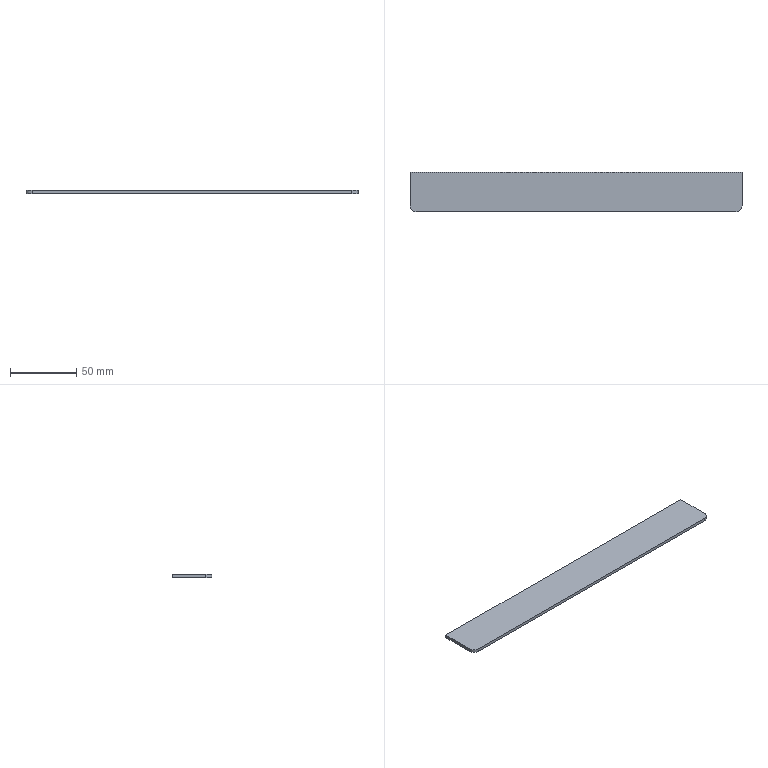Part | STEP file | [04]-7 | 1 solid | 8 faces | box 250 x 30 x 2.3 mm | volume 17229 mm3 | plane 6 | cylinder 2 | commonest cylinder face diameters 9.2 x2
STEP:
#1=CARTESIAN_POINT('',(0.,0.,0.));
#2=DIRECTION('',(0.,0.,1.));
#3=DIRECTION('',(1.,0.,0.));
#4=AXIS2_PLACEMENT_3D('',#1,#2,#3);
#5=CARTESIAN_POINT('',(0.,-25.4,0.));
#6=VERTEX_POINT('',#5);
#7=CARTESIAN_POINT('',(0.,0.,0.));
#8=VERTEX_POINT('',#7);
#9=CARTESIAN_POINT('',(0.,-15.,0.));
#10=DIRECTION('',(0.,1.,0.));
#11=VECTOR('',#10,1.);
#12=LINE('',#9,#11);
#13=CARTESIAN_POINT('',(125.,-15.,0.));
#14=DIRECTION('',(0.,0.,-1.));
#15=DIRECTION('',(-1.,0.,0.));
#16=AXIS2_PLACEMENT_3D('',#13,#14,#15);
#17=PLANE('',#16);
#18=CARTESIAN_POINT('',(125.,0.));
#19=DIRECTION('',(0.,1.));
#20=VECTOR('',#19,1.);
#21=LINE('',#18,#20);
#22=(GEOMETRIC_REPRESENTATION_CONTEXT(2)PARAMETRIC_REPRESENTATION_CONTEXT()REPRESENTATION_CONTEXT('',''));
#23=DEFINITIONAL_REPRESENTATION('',(#21),#22);
#24=PCURVE('',#17,#23);
#25=CARTESIAN_POINT('',(0.,-15.,2.3));
#26=DIRECTION('',(-1.,0.,0.));
#27=DIRECTION('',(0.,0.,1.));
#28=AXIS2_PLACEMENT_3D('',#25,#26,#27);
#29=PLANE('',#28);
#30=CARTESIAN_POINT('',(-2.3,0.));
#31=DIRECTION('',(0.,1.));
#32=VECTOR('',#31,1.);
#33=LINE('',#30,#32);
#34=(GEOMETRIC_REPRESENTATION_CONTEXT(2)PARAMETRIC_REPRESENTATION_CONTEXT()REPRESENTATION_CONTEXT('',''));
#35=DEFINITIONAL_REPRESENTATION('',(#33),#34);
#36=PCURVE('',#29,#35);
#37=SURFACE_CURVE('',#12,(#24,#36),.PCURVE_S1.);
#38=EDGE_CURVE('',#6,#8,#37,.T.);
#39=ORIENTED_EDGE('',*,*,#38,.T.);
#40=CARTESIAN_POINT('',(250.,0.,0.));
#41=VERTEX_POINT('',#40);
#42=CARTESIAN_POINT('',(125.,0.,0.));
#43=DIRECTION('',(1.,0.,0.));
#44=VECTOR('',#43,1.);
#45=LINE('',#42,#44);
#46=CARTESIAN_POINT('',(0.,15.));
#47=DIRECTION('',(-1.,0.));
#48=VECTOR('',#47,1.);
#49=LINE('',#46,#48);
#50=(GEOMETRIC_REPRESENTATION_CONTEXT(2)PARAMETRIC_REPRESENTATION_CONTEXT()REPRESENTATION_CONTEXT('',''));
#51=DEFINITIONAL_REPRESENTATION('',(#49),#50);
#52=PCURVE('',#17,#51);
#53=CARTESIAN_POINT('',(125.,0.,2.3));
#54=DIRECTION('',(0.,1.,0.));
#55=DIRECTION('',(0.,0.,1.));
#56=AXIS2_PLACEMENT_3D('',#53,#54,#55);
#57=PLANE('',#56);
#58=CARTESIAN_POINT('',(-2.3,0.));
#59=DIRECTION('',(0.,1.));
#60=VECTOR('',#59,1.);
#61=LINE('',#58,#60);
#62=(GEOMETRIC_REPRESENTATION_CONTEXT(2)PARAMETRIC_REPRESENTATION_CONTEXT()REPRESENTATION_CONTEXT('',''));
#63=DEFINITIONAL_REPRESENTATION('',(#61),#62);
#64=PCURVE('',#57,#63);
#65=SURFACE_CURVE('',#45,(#52,#64),.PCURVE_S1.);
#66=EDGE_CURVE('',#8,#41,#65,.T.);
#67=ORIENTED_EDGE('',*,*,#66,.T.);
#68=CARTESIAN_POINT('',(250.,-25.4,0.));
#69=VERTEX_POINT('',#68);
#70=CARTESIAN_POINT('',(250.,-15.,0.));
#71=DIRECTION('',(0.,-1.,0.));
#72=VECTOR('',#71,1.);
#73=LINE('',#70,#72);
#74=CARTESIAN_POINT('',(-125.,0.));
#75=DIRECTION('',(0.,-1.));
#76=VECTOR('',#75,1.);
#77=LINE('',#74,#76);
#78=(GEOMETRIC_REPRESENTATION_CONTEXT(2)PARAMETRIC_REPRESENTATION_CONTEXT()REPRESENTATION_CONTEXT('',''));
#79=DEFINITIONAL_REPRESENTATION('',(#77),#78);
#80=PCURVE('',#17,#79);
#81=CARTESIAN_POINT('',(250.,-15.,2.3));
#82=DIRECTION('',(1.,0.,0.));
#83=DIRECTION('',(0.,0.,-1.));
#84=AXIS2_PLACEMENT_3D('',#81,#82,#83);
#85=PLANE('',#84);
#86=CARTESIAN_POINT('',(2.3,0.));
#87=DIRECTION('',(0.,-1.));
#88=VECTOR('',#87,1.);
#89=LINE('',#86,#88);
#90=(GEOMETRIC_REPRESENTATION_CONTEXT(2)PARAMETRIC_REPRESENTATION_CONTEXT()REPRESENTATION_CONTEXT('',''));
#91=DEFINITIONAL_REPRESENTATION('',(#89),#90);
#92=PCURVE('',#85,#91);
#93=SURFACE_CURVE('',#73,(#80,#92),.PCURVE_S1.);
#94=EDGE_CURVE('',#41,#69,#93,.T.);
#95=ORIENTED_EDGE('',*,*,#94,.T.);
#96=CARTESIAN_POINT('',(245.4,-30.,0.));
#97=VERTEX_POINT('',#96);
#98=CARTESIAN_POINT('',(245.4,-25.4,0.));
#99=DIRECTION('',(0.,0.,1.));
#100=DIRECTION('',(-1.,0.,0.));
#101=AXIS2_PLACEMENT_3D('',#98,#99,#100);
#102=CIRCLE('',#101,4.6);
#103=CARTESIAN_POINT('',(-115.8,-10.4));
#104=CARTESIAN_POINT('',(-115.8,-18.367));
#105=CARTESIAN_POINT('',(-122.7,-14.384));
#106=CARTESIAN_POINT('',(-129.6,-10.4));
#107=CARTESIAN_POINT('',(-122.7,-6.416));
#108=CARTESIAN_POINT('',(-115.8,-2.433));
#109=CARTESIAN_POINT('',(-115.8,-10.4));
#110=(BOUNDED_CURVE()B_SPLINE_CURVE(2,(#103,#104,#105,#106,#107,#108,#109),.UNSPECIFIED.,.T.,.F.)B_SPLINE_CURVE_WITH_KNOTS((1,2,2,2,2,1),(-2.094,0.,2.094,4.189,6.283,8.378),.UNSPECIFIED.)CURVE()GEOMETRIC_REPRESENTATION_ITEM()RATIONAL_B_SPLINE_CURVE((1.,0.5,1.,0.5,1.,0.5,1.))REPRESENTATION_ITEM(''));
#111=(GEOMETRIC_REPRESENTATION_CONTEXT(2)PARAMETRIC_REPRESENTATION_CONTEXT()REPRESENTATION_CONTEXT('',''));
#112=DEFINITIONAL_REPRESENTATION('',(#110),#111);
#113=PCURVE('',#17,#112);
#114=CARTESIAN_POINT('',(245.4,-25.4,2.3));
#115=DIRECTION('',(0.,0.,-1.));
#116=DIRECTION('',(-1.,0.,0.));
#117=AXIS2_PLACEMENT_3D('',#114,#115,#116);
#118=CYLINDRICAL_SURFACE('',#117,4.6);
#119=CARTESIAN_POINT('',(6.283,2.3));
#120=DIRECTION('',(-1.,0.));
#121=VECTOR('',#120,1.);
#122=LINE('',#119,#121);
#123=(GEOMETRIC_REPRESENTATION_CONTEXT(2)PARAMETRIC_REPRESENTATION_CONTEXT()REPRESENTATION_CONTEXT('',''));
#124=DEFINITIONAL_REPRESENTATION('',(#122),#123);
#125=PCURVE('',#118,#124);
#126=SURFACE_CURVE('',#102,(#113,#125),.PCURVE_S1.);
#127=EDGE_CURVE('',#97,#69,#126,.T.);
#128=ORIENTED_EDGE('',*,*,#127,.F.);
#129=CARTESIAN_POINT('',(4.6,-30.,0.));
#130=VERTEX_POINT('',#129);
#131=CARTESIAN_POINT('',(125.,-30.,0.));
#132=DIRECTION('',(-1.,0.,0.));
#133=VECTOR('',#132,1.);
#134=LINE('',#131,#133);
#135=CARTESIAN_POINT('',(0.,-15.));
#136=DIRECTION('',(1.,0.));
#137=VECTOR('',#136,1.);
#138=LINE('',#135,#137);
#139=(GEOMETRIC_REPRESENTATION_CONTEXT(2)PARAMETRIC_REPRESENTATION_CONTEXT()REPRESENTATION_CONTEXT('',''));
#140=DEFINITIONAL_REPRESENTATION('',(#138),#139);
#141=PCURVE('',#17,#140);
#142=CARTESIAN_POINT('',(125.,-30.,2.3));
#143=DIRECTION('',(0.,-1.,0.));
#144=DIRECTION('',(0.,0.,-1.));
#145=AXIS2_PLACEMENT_3D('',#142,#143,#144);
#146=PLANE('',#145);
#147=CARTESIAN_POINT('',(2.3,0.));
#148=DIRECTION('',(0.,-1.));
#149=VECTOR('',#148,1.);
#150=LINE('',#147,#149);
#151=(GEOMETRIC_REPRESENTATION_CONTEXT(2)PARAMETRIC_REPRESENTATION_CONTEXT()REPRESENTATION_CONTEXT('',''));
#152=DEFINITIONAL_REPRESENTATION('',(#150),#151);
#153=PCURVE('',#146,#152);
#154=SURFACE_CURVE('',#134,(#141,#153),.PCURVE_S1.);
#155=EDGE_CURVE('',#97,#130,#154,.T.);
#156=ORIENTED_EDGE('',*,*,#155,.T.);
#157=CARTESIAN_POINT('',(4.6,-25.4,0.));
#158=DIRECTION('',(0.,0.,1.));
#159=DIRECTION('',(-1.,0.,0.));
#160=AXIS2_PLACEMENT_3D('',#157,#158,#159);
#161=CIRCLE('',#160,4.6);
#162=CARTESIAN_POINT('',(125.,-10.4));
#163=CARTESIAN_POINT('',(125.,-18.367));
#164=CARTESIAN_POINT('',(118.1,-14.384));
#165=CARTESIAN_POINT('',(111.2,-10.4));
#166=CARTESIAN_POINT('',(118.1,-6.416));
#167=CARTESIAN_POINT('',(125.,-2.433));
#168=CARTESIAN_POINT('',(125.,-10.4));
#169=(BOUNDED_CURVE()B_SPLINE_CURVE(2,(#162,#163,#164,#165,#166,#167,#168),.UNSPECIFIED.,.T.,.F.)B_SPLINE_CURVE_WITH_KNOTS((1,2,2,2,2,1),(-2.094,0.,2.094,4.189,6.283,8.378),.UNSPECIFIED.)CURVE()GEOMETRIC_REPRESENTATION_ITEM()RATIONAL_B_SPLINE_CURVE((1.,0.5,1.,0.5,1.,0.5,1.))REPRESENTATION_ITEM(''));
#170=(GEOMETRIC_REPRESENTATION_CONTEXT(2)PARAMETRIC_REPRESENTATION_CONTEXT()REPRESENTATION_CONTEXT('',''));
#171=DEFINITIONAL_REPRESENTATION('',(#169),#170);
#172=PCURVE('',#17,#171);
#173=CARTESIAN_POINT('',(4.6,-25.4,2.3));
#174=DIRECTION('',(0.,0.,-1.));
#175=DIRECTION('',(-1.,0.,0.));
#176=AXIS2_PLACEMENT_3D('',#173,#174,#175);
#177=CYLINDRICAL_SURFACE('',#176,4.6);
#178=CARTESIAN_POINT('',(6.283,2.3));
#179=DIRECTION('',(-1.,0.));
#180=VECTOR('',#179,1.);
#181=LINE('',#178,#180);
#182=(GEOMETRIC_REPRESENTATION_CONTEXT(2)PARAMETRIC_REPRESENTATION_CONTEXT()REPRESENTATION_CONTEXT('',''));
#183=DEFINITIONAL_REPRESENTATION('',(#181),#182);
#184=PCURVE('',#177,#183);
#185=SURFACE_CURVE('',#161,(#172,#184),.PCURVE_S1.);
#186=EDGE_CURVE('',#6,#130,#185,.T.);
#187=ORIENTED_EDGE('',*,*,#186,.F.);
#188=EDGE_LOOP('',(#39,#67,#95,#128,#156,#187));
#189=FACE_BOUND('',#188,.T.);
#190=ADVANCED_FACE('',(#189),#17,.T.);
#191=CARTESIAN_POINT('',(0.,0.,2.3));
#192=VERTEX_POINT('',#191);
#193=CARTESIAN_POINT('',(0.,0.,2.3));
#194=DIRECTION('',(0.,0.,-1.));
#195=VECTOR('',#194,1.);
#196=LINE('',#193,#195);
#197=CARTESIAN_POINT('',(0.,-125.));
#198=DIRECTION('',(-1.,0.));
#199=VECTOR('',#198,1.);
#200=LINE('',#197,#199);
#201=(GEOMETRIC_REPRESENTATION_CONTEXT(2)PARAMETRIC_REPRESENTATION_CONTEXT()REPRESENTATION_CONTEXT('',''));
#202=DEFINITIONAL_REPRESENTATION('',(#200),#201);
#203=PCURVE('',#57,#202);
#204=CARTESIAN_POINT('',(0.,15.));
#205=DIRECTION('',(-1.,0.));
#206=VECTOR('',#205,1.);
#207=LINE('',#204,#206);
#208=(GEOMETRIC_REPRESENTATION_CONTEXT(2)PARAMETRIC_REPRESENTATION_CONTEXT()REPRESENTATION_CONTEXT('',''));
#209=DEFINITIONAL_REPRESENTATION('',(#207),#208);
#210=PCURVE('',#29,#209);
#211=SURFACE_CURVE('',#196,(#203,#210),.PCURVE_S1.);
#212=EDGE_CURVE('',#192,#8,#211,.T.);
#213=ORIENTED_EDGE('',*,*,#212,.F.);
#214=CARTESIAN_POINT('',(250.,0.,2.3));
#215=VERTEX_POINT('',#214);
#216=CARTESIAN_POINT('',(125.,0.,2.3));
#217=DIRECTION('',(-1.,0.,0.));
#218=VECTOR('',#217,1.);
#219=LINE('',#216,#218);
#220=CARTESIAN_POINT('',(0.,0.));
#221=DIRECTION('',(0.,-1.));
#222=VECTOR('',#221,1.);
#223=LINE('',#220,#222);
#224=(GEOMETRIC_REPRESENTATION_CONTEXT(2)PARAMETRIC_REPRESENTATION_CONTEXT()REPRESENTATION_CONTEXT('',''));
#225=DEFINITIONAL_REPRESENTATION('',(#223),#224);
#226=PCURVE('',#57,#225);
#227=CARTESIAN_POINT('',(125.,-15.,2.3));
#228=DIRECTION('',(0.,0.,1.));
#229=DIRECTION('',(1.,0.,0.));
#230=AXIS2_PLACEMENT_3D('',#227,#228,#229);
#231=PLANE('',#230);
#232=CARTESIAN_POINT('',(0.,15.));
#233=DIRECTION('',(-1.,0.));
#234=VECTOR('',#233,1.);
#235=LINE('',#232,#234);
#236=(GEOMETRIC_REPRESENTATION_CONTEXT(2)PARAMETRIC_REPRESENTATION_CONTEXT()REPRESENTATION_CONTEXT('',''));
#237=DEFINITIONAL_REPRESENTATION('',(#235),#236);
#238=PCURVE('',#231,#237);
#239=SURFACE_CURVE('',#219,(#226,#238),.PCURVE_S1.);
#240=EDGE_CURVE('',#215,#192,#239,.T.);
#241=ORIENTED_EDGE('',*,*,#240,.F.);
#242=CARTESIAN_POINT('',(250.,0.,2.3));
#243=DIRECTION('',(0.,0.,-1.));
#244=VECTOR('',#243,1.);
#245=LINE('',#242,#244);
#246=CARTESIAN_POINT('',(0.,125.));
#247=DIRECTION('',(-1.,0.));
#248=VECTOR('',#247,1.);
#249=LINE('',#246,#248);
#250=(GEOMETRIC_REPRESENTATION_CONTEXT(2)PARAMETRIC_REPRESENTATION_CONTEXT()REPRESENTATION_CONTEXT('',''));
#251=DEFINITIONAL_REPRESENTATION('',(#249),#250);
#252=PCURVE('',#57,#251);
#253=CARTESIAN_POINT('',(0.,15.));
#254=DIRECTION('',(1.,0.));
#255=VECTOR('',#254,1.);
#256=LINE('',#253,#255);
#257=(GEOMETRIC_REPRESENTATION_CONTEXT(2)PARAMETRIC_REPRESENTATION_CONTEXT()REPRESENTATION_CONTEXT('',''));
#258=DEFINITIONAL_REPRESENTATION('',(#256),#257);
#259=PCURVE('',#85,#258);
#260=SURFACE_CURVE('',#245,(#252,#259),.PCURVE_S1.);
#261=EDGE_CURVE('',#215,#41,#260,.T.);
#262=ORIENTED_EDGE('',*,*,#261,.T.);
#263=ORIENTED_EDGE('',*,*,#66,.F.);
#264=EDGE_LOOP('',(#213,#241,#262,#263));
#265=FACE_BOUND('',#264,.T.);
#266=ADVANCED_FACE('',(#265),#57,.T.);
#267=ORIENTED_EDGE('',*,*,#94,.F.);
#268=ORIENTED_EDGE('',*,*,#261,.F.);
#269=CARTESIAN_POINT('',(250.,-25.4,2.3));
#270=VERTEX_POINT('',#269);
#271=CARTESIAN_POINT('',(250.,-15.,2.3));
#272=DIRECTION('',(0.,1.,0.));
#273=VECTOR('',#272,1.);
#274=LINE('',#271,#273);
#275=CARTESIAN_POINT('',(0.,0.));
#276=DIRECTION('',(0.,1.));
#277=VECTOR('',#276,1.);
#278=LINE('',#275,#277);
#279=(GEOMETRIC_REPRESENTATION_CONTEXT(2)PARAMETRIC_REPRESENTATION_CONTEXT()REPRESENTATION_CONTEXT('',''));
#280=DEFINITIONAL_REPRESENTATION('',(#278),#279);
#281=PCURVE('',#85,#280);
#282=CARTESIAN_POINT('',(125.,0.));
#283=DIRECTION('',(0.,1.));
#284=VECTOR('',#283,1.);
#285=LINE('',#282,#284);
#286=(GEOMETRIC_REPRESENTATION_CONTEXT(2)PARAMETRIC_REPRESENTATION_CONTEXT()REPRESENTATION_CONTEXT('',''));
#287=DEFINITIONAL_REPRESENTATION('',(#285),#286);
#288=PCURVE('',#231,#287);
#289=SURFACE_CURVE('',#274,(#281,#288),.PCURVE_S1.);
#290=EDGE_CURVE('',#270,#215,#289,.T.);
#291=ORIENTED_EDGE('',*,*,#290,.F.);
#292=CARTESIAN_POINT('',(250.,-25.4,2.3));
#293=DIRECTION('',(0.,0.,1.));
#294=VECTOR('',#293,1.);
#295=LINE('',#292,#294);
#296=CARTESIAN_POINT('',(0.,-10.4));
#297=DIRECTION('',(-1.,0.));
#298=VECTOR('',#297,1.);
#299=LINE('',#296,#298);
#300=(GEOMETRIC_REPRESENTATION_CONTEXT(2)PARAMETRIC_REPRESENTATION_CONTEXT()REPRESENTATION_CONTEXT('',''));
#301=DEFINITIONAL_REPRESENTATION('',(#299),#300);
#302=PCURVE('',#85,#301);
#303=CARTESIAN_POINT('',(3.142,0.));
#304=DIRECTION('',(0.,-1.));
#305=VECTOR('',#304,1.);
#306=LINE('',#303,#305);
#307=(GEOMETRIC_REPRESENTATION_CONTEXT(2)PARAMETRIC_REPRESENTATION_CONTEXT()REPRESENTATION_CONTEXT('',''));
#308=DEFINITIONAL_REPRESENTATION('',(#306),#307);
#309=PCURVE('',#118,#308);
#310=SURFACE_CURVE('',#295,(#302,#309),.PCURVE_S1.);
#311=EDGE_CURVE('',#69,#270,#310,.T.);
#312=ORIENTED_EDGE('',*,*,#311,.F.);
#313=EDGE_LOOP('',(#267,#268,#291,#312));
#314=FACE_BOUND('',#313,.T.);
#315=ADVANCED_FACE('',(#314),#85,.T.);
#316=ORIENTED_EDGE('',*,*,#155,.F.);
#317=CARTESIAN_POINT('',(245.4,-30.,2.3));
#318=VERTEX_POINT('',#317);
#319=CARTESIAN_POINT('',(245.4,-30.,2.3));
#320=DIRECTION('',(0.,0.,-1.));
#321=VECTOR('',#320,1.);
#322=LINE('',#319,#321);
#323=CARTESIAN_POINT('',(0.,120.4));
#324=DIRECTION('',(1.,0.));
#325=VECTOR('',#324,1.);
#326=LINE('',#323,#325);
#327=(GEOMETRIC_REPRESENTATION_CONTEXT(2)PARAMETRIC_REPRESENTATION_CONTEXT()REPRESENTATION_CONTEXT('',''));
#328=DEFINITIONAL_REPRESENTATION('',(#326),#327);
#329=PCURVE('',#146,#328);
#330=CARTESIAN_POINT('',(4.712,0.));
#331=DIRECTION('',(0.,1.));
#332=VECTOR('',#331,1.);
#333=LINE('',#330,#332);
#334=(GEOMETRIC_REPRESENTATION_CONTEXT(2)PARAMETRIC_REPRESENTATION_CONTEXT()REPRESENTATION_CONTEXT('',''));
#335=DEFINITIONAL_REPRESENTATION('',(#333),#334);
#336=PCURVE('',#118,#335);
#337=SURFACE_CURVE('',#322,(#329,#336),.PCURVE_S1.);
#338=EDGE_CURVE('',#318,#97,#337,.T.);
#339=ORIENTED_EDGE('',*,*,#338,.F.);
#340=CARTESIAN_POINT('',(4.6,-30.,2.3));
#341=VERTEX_POINT('',#340);
#342=CARTESIAN_POINT('',(125.,-30.,2.3));
#343=DIRECTION('',(1.,0.,0.));
#344=VECTOR('',#343,1.);
#345=LINE('',#342,#344);
#346=CARTESIAN_POINT('',(0.,0.));
#347=DIRECTION('',(0.,1.));
#348=VECTOR('',#347,1.);
#349=LINE('',#346,#348);
#350=(GEOMETRIC_REPRESENTATION_CONTEXT(2)PARAMETRIC_REPRESENTATION_CONTEXT()REPRESENTATION_CONTEXT('',''));
#351=DEFINITIONAL_REPRESENTATION('',(#349),#350);
#352=PCURVE('',#146,#351);
#353=CARTESIAN_POINT('',(0.,-15.));
#354=DIRECTION('',(1.,0.));
#355=VECTOR('',#354,1.);
#356=LINE('',#353,#355);
#357=(GEOMETRIC_REPRESENTATION_CONTEXT(2)PARAMETRIC_REPRESENTATION_CONTEXT()REPRESENTATION_CONTEXT('',''));
#358=DEFINITIONAL_REPRESENTATION('',(#356),#357);
#359=PCURVE('',#231,#358);
#360=SURFACE_CURVE('',#345,(#352,#359),.PCURVE_S1.);
#361=EDGE_CURVE('',#341,#318,#360,.T.);
#362=ORIENTED_EDGE('',*,*,#361,.F.);
#363=CARTESIAN_POINT('',(4.6,-30.,2.3));
#364=DIRECTION('',(0.,0.,1.));
#365=VECTOR('',#364,1.);
#366=LINE('',#363,#365);
#367=CARTESIAN_POINT('',(0.,-120.4));
#368=DIRECTION('',(-1.,0.));
#369=VECTOR('',#368,1.);
#370=LINE('',#367,#369);
#371=(GEOMETRIC_REPRESENTATION_CONTEXT(2)PARAMETRIC_REPRESENTATION_CONTEXT()REPRESENTATION_CONTEXT('',''));
#372=DEFINITIONAL_REPRESENTATION('',(#370),#371);
#373=PCURVE('',#146,#372);
#374=CARTESIAN_POINT('',(4.712,0.));
#375=DIRECTION('',(0.,-1.));
#376=VECTOR('',#375,1.);
#377=LINE('',#374,#376);
#378=(GEOMETRIC_REPRESENTATION_CONTEXT(2)PARAMETRIC_REPRESENTATION_CONTEXT()REPRESENTATION_CONTEXT('',''));
#379=DEFINITIONAL_REPRESENTATION('',(#377),#378);
#380=PCURVE('',#177,#379);
#381=SURFACE_CURVE('',#366,(#373,#380),.PCURVE_S1.);
#382=EDGE_CURVE('',#130,#341,#381,.T.);
#383=ORIENTED_EDGE('',*,*,#382,.F.);
#384=EDGE_LOOP('',(#316,#339,#362,#383));
#385=FACE_BOUND('',#384,.T.);
#386=ADVANCED_FACE('',(#385),#146,.T.);
#387=ORIENTED_EDGE('',*,*,#361,.T.);
#388=CARTESIAN_POINT('',(245.4,-25.4,2.3));
#389=DIRECTION('',(0.,0.,-1.));
#390=DIRECTION('',(1.,0.,0.));
#391=AXIS2_PLACEMENT_3D('',#388,#389,#390);
#392=CIRCLE('',#391,4.6);
#393=CARTESIAN_POINT('',(125.,-10.4));
#394=CARTESIAN_POINT('',(125.,-18.367));
#395=CARTESIAN_POINT('',(118.1,-14.384));
#396=CARTESIAN_POINT('',(111.2,-10.4));
#397=CARTESIAN_POINT('',(118.1,-6.416));
#398=CARTESIAN_POINT('',(125.,-2.433));
#399=CARTESIAN_POINT('',(125.,-10.4));
#400=(BOUNDED_CURVE()B_SPLINE_CURVE(2,(#393,#394,#395,#396,#397,#398,#399),.UNSPECIFIED.,.T.,.F.)B_SPLINE_CURVE_WITH_KNOTS((1,2,2,2,2,1),(-2.094,0.,2.094,4.189,6.283,8.378),.UNSPECIFIED.)CURVE()GEOMETRIC_REPRESENTATION_ITEM()RATIONAL_B_SPLINE_CURVE((1.,0.5,1.,0.5,1.,0.5,1.))REPRESENTATION_ITEM(''));
#401=(GEOMETRIC_REPRESENTATION_CONTEXT(2)PARAMETRIC_REPRESENTATION_CONTEXT()REPRESENTATION_CONTEXT('',''));
#402=DEFINITIONAL_REPRESENTATION('',(#400),#401);
#403=PCURVE('',#231,#402);
#404=CARTESIAN_POINT('',(3.142,0.));
#405=DIRECTION('',(1.,0.));
#406=VECTOR('',#405,1.);
#407=LINE('',#404,#406);
#408=(GEOMETRIC_REPRESENTATION_CONTEXT(2)PARAMETRIC_REPRESENTATION_CONTEXT()REPRESENTATION_CONTEXT('',''));
#409=DEFINITIONAL_REPRESENTATION('',(#407),#408);
#410=PCURVE('',#118,#409);
#411=SURFACE_CURVE('',#392,(#403,#410),.PCURVE_S1.);
#412=EDGE_CURVE('',#270,#318,#411,.T.);
#413=ORIENTED_EDGE('',*,*,#412,.F.);
#414=ORIENTED_EDGE('',*,*,#290,.T.);
#415=ORIENTED_EDGE('',*,*,#240,.T.);
#416=CARTESIAN_POINT('',(0.,-25.4,2.3));
#417=VERTEX_POINT('',#416);
#418=CARTESIAN_POINT('',(0.,-15.,2.3));
#419=DIRECTION('',(0.,-1.,0.));
#420=VECTOR('',#419,1.);
#421=LINE('',#418,#420);
#422=CARTESIAN_POINT('',(-125.,0.));
#423=DIRECTION('',(0.,-1.));
#424=VECTOR('',#423,1.);
#425=LINE('',#422,#424);
#426=(GEOMETRIC_REPRESENTATION_CONTEXT(2)PARAMETRIC_REPRESENTATION_CONTEXT()REPRESENTATION_CONTEXT('',''));
#427=DEFINITIONAL_REPRESENTATION('',(#425),#426);
#428=PCURVE('',#231,#427);
#429=CARTESIAN_POINT('',(0.,0.));
#430=DIRECTION('',(0.,-1.));
#431=VECTOR('',#430,1.);
#432=LINE('',#429,#431);
#433=(GEOMETRIC_REPRESENTATION_CONTEXT(2)PARAMETRIC_REPRESENTATION_CONTEXT()REPRESENTATION_CONTEXT('',''));
#434=DEFINITIONAL_REPRESENTATION('',(#432),#433);
#435=PCURVE('',#29,#434);
#436=SURFACE_CURVE('',#421,(#428,#435),.PCURVE_S1.);
#437=EDGE_CURVE('',#192,#417,#436,.T.);
#438=ORIENTED_EDGE('',*,*,#437,.T.);
#439=CARTESIAN_POINT('',(4.6,-25.4,2.3));
#440=DIRECTION('',(0.,0.,-1.));
#441=DIRECTION('',(1.,0.,0.));
#442=AXIS2_PLACEMENT_3D('',#439,#440,#441);
#443=CIRCLE('',#442,4.6);
#444=CARTESIAN_POINT('',(-115.8,-10.4));
#445=CARTESIAN_POINT('',(-115.8,-18.367));
#446=CARTESIAN_POINT('',(-122.7,-14.384));
#447=CARTESIAN_POINT('',(-129.6,-10.4));
#448=CARTESIAN_POINT('',(-122.7,-6.416));
#449=CARTESIAN_POINT('',(-115.8,-2.433));
#450=CARTESIAN_POINT('',(-115.8,-10.4));
#451=(BOUNDED_CURVE()B_SPLINE_CURVE(2,(#444,#445,#446,#447,#448,#449,#450),.UNSPECIFIED.,.T.,.F.)B_SPLINE_CURVE_WITH_KNOTS((1,2,2,2,2,1),(-2.094,0.,2.094,4.189,6.283,8.378),.UNSPECIFIED.)CURVE()GEOMETRIC_REPRESENTATION_ITEM()RATIONAL_B_SPLINE_CURVE((1.,0.5,1.,0.5,1.,0.5,1.))REPRESENTATION_ITEM(''));
#452=(GEOMETRIC_REPRESENTATION_CONTEXT(2)PARAMETRIC_REPRESENTATION_CONTEXT()REPRESENTATION_CONTEXT('',''));
#453=DEFINITIONAL_REPRESENTATION('',(#451),#452);
#454=PCURVE('',#231,#453);
#455=CARTESIAN_POINT('',(3.142,0.));
#456=DIRECTION('',(1.,0.));
#457=VECTOR('',#456,1.);
#458=LINE('',#455,#457);
#459=(GEOMETRIC_REPRESENTATION_CONTEXT(2)PARAMETRIC_REPRESENTATION_CONTEXT()REPRESENTATION_CONTEXT('',''));
#460=DEFINITIONAL_REPRESENTATION('',(#458),#459);
#461=PCURVE('',#177,#460);
#462=SURFACE_CURVE('',#443,(#454,#461),.PCURVE_S1.);
#463=EDGE_CURVE('',#341,#417,#462,.T.);
#464=ORIENTED_EDGE('',*,*,#463,.F.);
#465=EDGE_LOOP('',(#387,#413,#414,#415,#438,#464));
#466=FACE_BOUND('',#465,.T.);
#467=ADVANCED_FACE('',(#466),#231,.T.);
#468=ORIENTED_EDGE('',*,*,#437,.F.);
#469=ORIENTED_EDGE('',*,*,#212,.T.);
#470=ORIENTED_EDGE('',*,*,#38,.F.);
#471=CARTESIAN_POINT('',(0.,-25.4,2.3));
#472=DIRECTION('',(0.,0.,-1.));
#473=VECTOR('',#472,1.);
#474=LINE('',#471,#473);
#475=CARTESIAN_POINT('',(0.,-10.4));
#476=DIRECTION('',(-1.,0.));
#477=VECTOR('',#476,1.);
#478=LINE('',#475,#477);
#479=(GEOMETRIC_REPRESENTATION_CONTEXT(2)PARAMETRIC_REPRESENTATION_CONTEXT()REPRESENTATION_CONTEXT('',''));
#480=DEFINITIONAL_REPRESENTATION('',(#478),#479);
#481=PCURVE('',#29,#480);
#482=CARTESIAN_POINT('',(6.283,0.));
#483=DIRECTION('',(0.,1.));
#484=VECTOR('',#483,1.);
#485=LINE('',#482,#484);
#486=(GEOMETRIC_REPRESENTATION_CONTEXT(2)PARAMETRIC_REPRESENTATION_CONTEXT()REPRESENTATION_CONTEXT('',''));
#487=DEFINITIONAL_REPRESENTATION('',(#485),#486);
#488=PCURVE('',#177,#487);
#489=SURFACE_CURVE('',#474,(#481,#488),.PCURVE_S1.);
#490=EDGE_CURVE('',#417,#6,#489,.T.);
#491=ORIENTED_EDGE('',*,*,#490,.F.);
#492=EDGE_LOOP('',(#468,#469,#470,#491));
#493=FACE_BOUND('',#492,.T.);
#494=ADVANCED_FACE('',(#493),#29,.T.);
#495=ORIENTED_EDGE('',*,*,#412,.T.);
#496=ORIENTED_EDGE('',*,*,#338,.T.);
#497=ORIENTED_EDGE('',*,*,#127,.T.);
#498=ORIENTED_EDGE('',*,*,#311,.T.);
#499=EDGE_LOOP('',(#495,#496,#497,#498));
#500=FACE_BOUND('',#499,.T.);
#501=ADVANCED_FACE('',(#500),#118,.T.);
#502=ORIENTED_EDGE('',*,*,#463,.T.);
#503=ORIENTED_EDGE('',*,*,#490,.T.);
#504=ORIENTED_EDGE('',*,*,#186,.T.);
#505=ORIENTED_EDGE('',*,*,#382,.T.);
#506=EDGE_LOOP('',(#502,#503,#504,#505));
#507=FACE_BOUND('',#506,.T.);
#508=ADVANCED_FACE('',(#507),#177,.T.);
#509=CLOSED_SHELL('',(#190,#266,#315,#386,#467,#494,#501,#508));
#510=MANIFOLD_SOLID_BREP('',#509);
#511=(LENGTH_UNIT()NAMED_UNIT(*)SI_UNIT(.MILLI.,.METRE.));
#512=UNCERTAINTY_MEASURE_WITH_UNIT(LENGTH_MEASURE(0.0000001),#511,'','');
#513=(NAMED_UNIT(*)PLANE_ANGLE_UNIT()SI_UNIT($,.RADIAN.));
#514=(NAMED_UNIT(*)SI_UNIT($,.STERADIAN.)SOLID_ANGLE_UNIT());
#515=(GEOMETRIC_REPRESENTATION_CONTEXT(3)GLOBAL_UNCERTAINTY_ASSIGNED_CONTEXT((#512))GLOBAL_UNIT_ASSIGNED_CONTEXT((#511,#513,#514))REPRESENTATION_CONTEXT('',''));
#516=ADVANCED_BREP_SHAPE_REPRESENTATION('',(#4,#510),#515);